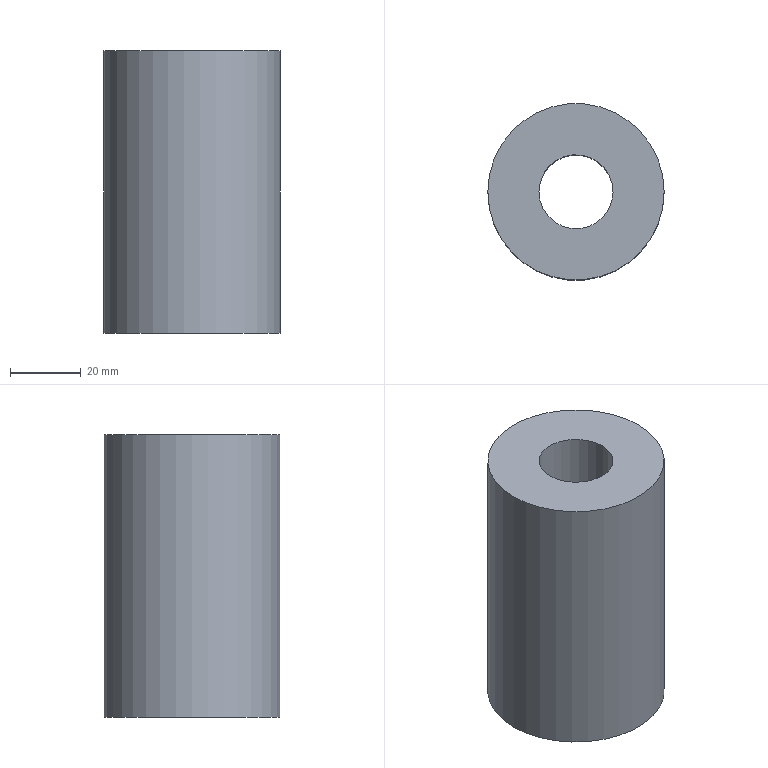Part | STEP file | SN10_014_002-02_TUBO | 1 solid | 4 faces | box 50 x 50 x 80 mm | volume 129371 mm3 | cylinder 2 | plane 2 | commonest cylinder face diameters 21 x1 50 x1
STEP:
#1=CARTESIAN_POINT('',(0.,0.,0.));
#2=DIRECTION('',(0.,0.,1.));
#3=DIRECTION('',(1.,0.,0.));
#4=AXIS2_PLACEMENT_3D('',#1,#2,#3);
#5=CARTESIAN_POINT('',(9.215,-5.034,92.5));
#6=VERTEX_POINT('',#5);
#7=CARTESIAN_POINT('',(0.,0.,92.5));
#8=DIRECTION('',(0.,0.,-1.));
#9=DIRECTION('',(1.,0.,0.));
#10=AXIS2_PLACEMENT_3D('',#7,#8,#9);
#11=CIRCLE('',#10,10.5);
#12=CARTESIAN_POINT('',(0.,0.,92.4));
#13=DIRECTION('',(0.,0.,-1.));
#14=DIRECTION('',(0.8776,-0.4794,0.));
#15=AXIS2_PLACEMENT_3D('',#12,#13,#14);
#16=CYLINDRICAL_SURFACE('',#15,10.5);
#17=CARTESIAN_POINT('',(-0.5,-0.1));
#18=DIRECTION('',(1.,0.));
#19=VECTOR('',#18,1.);
#20=LINE('',#17,#19);
#21=(GEOMETRIC_REPRESENTATION_CONTEXT(2)PARAMETRIC_REPRESENTATION_CONTEXT()REPRESENTATION_CONTEXT('',''));
#22=DEFINITIONAL_REPRESENTATION('',(#20),#21);
#23=PCURVE('',#16,#22);
#24=CARTESIAN_POINT('',(0.,0.,92.5));
#25=DIRECTION('',(0.,0.,-1.));
#26=DIRECTION('',(-1.,0.,0.));
#27=AXIS2_PLACEMENT_3D('',#24,#25,#26);
#28=PLANE('',#27);
#29=CARTESIAN_POINT('',(0.,0.));
#30=DIRECTION('',(-1.,0.));
#31=AXIS2_PLACEMENT_2D('',#29,#30);
#32=CIRCLE('',#31,10.5);
#33=(GEOMETRIC_REPRESENTATION_CONTEXT(2)PARAMETRIC_REPRESENTATION_CONTEXT()REPRESENTATION_CONTEXT('',''));
#34=DEFINITIONAL_REPRESENTATION('',(#32),#33);
#35=PCURVE('',#28,#34);
#36=SURFACE_CURVE('',#11,(#23,#35),.PCURVE_S1.);
#37=EDGE_CURVE('',#6,#6,#36,.T.);
#38=ORIENTED_EDGE('',*,*,#37,.T.);
#39=CARTESIAN_POINT('',(9.215,-5.034,12.5));
#40=VERTEX_POINT('',#39);
#41=CARTESIAN_POINT('',(9.215,-5.034,92.5));
#42=CARTESIAN_POINT('',(9.215,-5.034,12.5));
#43=B_SPLINE_CURVE_WITH_KNOTS('',1,(#41,#42),.UNSPECIFIED.,.F.,.F.,(2,2),(-0.1,79.9),.PIECEWISE_BEZIER_KNOTS.);
#44=CARTESIAN_POINT('',(6.283,0.));
#45=DIRECTION('',(0.,1.));
#46=VECTOR('',#45,1.);
#47=LINE('',#44,#46);
#48=(GEOMETRIC_REPRESENTATION_CONTEXT(2)PARAMETRIC_REPRESENTATION_CONTEXT()REPRESENTATION_CONTEXT('',''));
#49=DEFINITIONAL_REPRESENTATION('',(#47),#48);
#50=PCURVE('',#16,#49);
#51=CARTESIAN_POINT('',(0.,0.));
#52=DIRECTION('',(0.,1.));
#53=VECTOR('',#52,1.);
#54=LINE('',#51,#53);
#55=(GEOMETRIC_REPRESENTATION_CONTEXT(2)PARAMETRIC_REPRESENTATION_CONTEXT()REPRESENTATION_CONTEXT('',''));
#56=DEFINITIONAL_REPRESENTATION('',(#54),#55);
#57=PCURVE('',#16,#56);
#58=SEAM_CURVE('',#43,(#50,#57),.PCURVE_S1.);
#59=EDGE_CURVE('',#6,#40,#58,.T.);
#60=ORIENTED_EDGE('',*,*,#59,.T.);
#61=CARTESIAN_POINT('',(0.,0.,12.5));
#62=DIRECTION('',(0.,0.,-1.));
#63=DIRECTION('',(1.,0.,0.));
#64=AXIS2_PLACEMENT_3D('',#61,#62,#63);
#65=CIRCLE('',#64,10.5);
#66=CARTESIAN_POINT('',(-0.5,79.9));
#67=DIRECTION('',(1.,0.));
#68=VECTOR('',#67,1.);
#69=LINE('',#66,#68);
#70=(GEOMETRIC_REPRESENTATION_CONTEXT(2)PARAMETRIC_REPRESENTATION_CONTEXT()REPRESENTATION_CONTEXT('',''));
#71=DEFINITIONAL_REPRESENTATION('',(#69),#70);
#72=PCURVE('',#16,#71);
#73=CARTESIAN_POINT('',(0.,0.,12.5));
#74=DIRECTION('',(0.,0.,-1.));
#75=DIRECTION('',(-1.,0.,0.));
#76=AXIS2_PLACEMENT_3D('',#73,#74,#75);
#77=PLANE('',#76);
#78=CARTESIAN_POINT('',(0.,0.));
#79=DIRECTION('',(-1.,0.));
#80=AXIS2_PLACEMENT_2D('',#78,#79);
#81=CIRCLE('',#80,10.5);
#82=(GEOMETRIC_REPRESENTATION_CONTEXT(2)PARAMETRIC_REPRESENTATION_CONTEXT()REPRESENTATION_CONTEXT('',''));
#83=DEFINITIONAL_REPRESENTATION('',(#81),#82);
#84=PCURVE('',#77,#83);
#85=SURFACE_CURVE('',#65,(#72,#84),.PCURVE_S1.);
#86=EDGE_CURVE('',#40,#40,#85,.T.);
#87=ORIENTED_EDGE('',*,*,#86,.F.);
#88=ORIENTED_EDGE('',*,*,#59,.F.);
#89=EDGE_LOOP('',(#38,#60,#87,#88));
#90=FACE_BOUND('',#89,.F.);
#91=ADVANCED_FACE('',(#90),#16,.F.);
#92=CARTESIAN_POINT('',(25.,0.,12.5));
#93=VERTEX_POINT('',#92);
#94=CARTESIAN_POINT('',(0.,0.,12.5));
#95=DIRECTION('',(0.,0.,-1.));
#96=DIRECTION('',(1.,0.,0.));
#97=AXIS2_PLACEMENT_3D('',#94,#95,#96);
#98=CIRCLE('',#97,25.);
#99=CARTESIAN_POINT('',(0.,0.));
#100=DIRECTION('',(-1.,0.));
#101=AXIS2_PLACEMENT_2D('',#99,#100);
#102=CIRCLE('',#101,25.);
#103=(GEOMETRIC_REPRESENTATION_CONTEXT(2)PARAMETRIC_REPRESENTATION_CONTEXT()REPRESENTATION_CONTEXT('',''));
#104=DEFINITIONAL_REPRESENTATION('',(#102),#103);
#105=PCURVE('',#77,#104);
#106=CARTESIAN_POINT('',(0.,0.,52.5));
#107=DIRECTION('',(0.,0.,-1.));
#108=DIRECTION('',(1.,0.,0.));
#109=AXIS2_PLACEMENT_3D('',#106,#107,#108);
#110=CYLINDRICAL_SURFACE('',#109,25.);
#111=CARTESIAN_POINT('',(0.,40.));
#112=DIRECTION('',(1.,0.));
#113=VECTOR('',#112,1.);
#114=LINE('',#111,#113);
#115=(GEOMETRIC_REPRESENTATION_CONTEXT(2)PARAMETRIC_REPRESENTATION_CONTEXT()REPRESENTATION_CONTEXT('',''));
#116=DEFINITIONAL_REPRESENTATION('',(#114),#115);
#117=PCURVE('',#110,#116);
#118=SURFACE_CURVE('',#98,(#105,#117),.PCURVE_S1.);
#119=EDGE_CURVE('',#93,#93,#118,.T.);
#120=ORIENTED_EDGE('',*,*,#119,.T.);
#121=EDGE_LOOP('',(#120));
#122=FACE_BOUND('',#121,.T.);
#123=ORIENTED_EDGE('',*,*,#86,.F.);
#124=EDGE_LOOP('',(#123));
#125=FACE_BOUND('',#124,.T.);
#126=ADVANCED_FACE('',(#122,#125),#77,.T.);
#127=CARTESIAN_POINT('',(25.,0.,92.5));
#128=VERTEX_POINT('',#127);
#129=CARTESIAN_POINT('',(0.,0.,92.5));
#130=DIRECTION('',(0.,0.,-1.));
#131=DIRECTION('',(1.,0.,0.));
#132=AXIS2_PLACEMENT_3D('',#129,#130,#131);
#133=CIRCLE('',#132,25.);
#134=CARTESIAN_POINT('',(0.,-40.));
#135=DIRECTION('',(1.,0.));
#136=VECTOR('',#135,1.);
#137=LINE('',#134,#136);
#138=(GEOMETRIC_REPRESENTATION_CONTEXT(2)PARAMETRIC_REPRESENTATION_CONTEXT()REPRESENTATION_CONTEXT('',''));
#139=DEFINITIONAL_REPRESENTATION('',(#137),#138);
#140=PCURVE('',#110,#139);
#141=CARTESIAN_POINT('',(0.,0.));
#142=DIRECTION('',(-1.,0.));
#143=AXIS2_PLACEMENT_2D('',#141,#142);
#144=CIRCLE('',#143,25.);
#145=(GEOMETRIC_REPRESENTATION_CONTEXT(2)PARAMETRIC_REPRESENTATION_CONTEXT()REPRESENTATION_CONTEXT('',''));
#146=DEFINITIONAL_REPRESENTATION('',(#144),#145);
#147=PCURVE('',#28,#146);
#148=SURFACE_CURVE('',#133,(#140,#147),.PCURVE_S1.);
#149=EDGE_CURVE('',#128,#128,#148,.T.);
#150=ORIENTED_EDGE('',*,*,#149,.T.);
#151=CARTESIAN_POINT('',(25.,0.,92.5));
#152=CARTESIAN_POINT('',(25.,0.,12.5));
#153=B_SPLINE_CURVE_WITH_KNOTS('',1,(#151,#152),.UNSPECIFIED.,.F.,.F.,(2,2),(-40.,40.),.PIECEWISE_BEZIER_KNOTS.);
#154=CARTESIAN_POINT('',(6.283,0.));
#155=DIRECTION('',(0.,1.));
#156=VECTOR('',#155,1.);
#157=LINE('',#154,#156);
#158=(GEOMETRIC_REPRESENTATION_CONTEXT(2)PARAMETRIC_REPRESENTATION_CONTEXT()REPRESENTATION_CONTEXT('',''));
#159=DEFINITIONAL_REPRESENTATION('',(#157),#158);
#160=PCURVE('',#110,#159);
#161=CARTESIAN_POINT('',(0.,0.));
#162=DIRECTION('',(0.,1.));
#163=VECTOR('',#162,1.);
#164=LINE('',#161,#163);
#165=(GEOMETRIC_REPRESENTATION_CONTEXT(2)PARAMETRIC_REPRESENTATION_CONTEXT()REPRESENTATION_CONTEXT('',''));
#166=DEFINITIONAL_REPRESENTATION('',(#164),#165);
#167=PCURVE('',#110,#166);
#168=SEAM_CURVE('',#153,(#160,#167),.PCURVE_S1.);
#169=EDGE_CURVE('',#128,#93,#168,.T.);
#170=ORIENTED_EDGE('',*,*,#169,.T.);
#171=ORIENTED_EDGE('',*,*,#119,.F.);
#172=ORIENTED_EDGE('',*,*,#169,.F.);
#173=EDGE_LOOP('',(#150,#170,#171,#172));
#174=FACE_BOUND('',#173,.T.);
#175=ADVANCED_FACE('',(#174),#110,.T.);
#176=ORIENTED_EDGE('',*,*,#149,.F.);
#177=EDGE_LOOP('',(#176));
#178=FACE_BOUND('',#177,.T.);
#179=ORIENTED_EDGE('',*,*,#37,.T.);
#180=EDGE_LOOP('',(#179));
#181=FACE_BOUND('',#180,.T.);
#182=ADVANCED_FACE('',(#178,#181),#28,.F.);
#183=CLOSED_SHELL('',(#91,#126,#175,#182));
#184=MANIFOLD_SOLID_BREP('',#183);
#185=(LENGTH_UNIT()NAMED_UNIT(*)SI_UNIT(.MILLI.,.METRE.));
#186=UNCERTAINTY_MEASURE_WITH_UNIT(LENGTH_MEASURE(0.00001),#185,'','');
#187=(NAMED_UNIT(*)PLANE_ANGLE_UNIT()SI_UNIT($,.RADIAN.));
#188=(NAMED_UNIT(*)SI_UNIT($,.STERADIAN.)SOLID_ANGLE_UNIT());
#189=(GEOMETRIC_REPRESENTATION_CONTEXT(3)GLOBAL_UNCERTAINTY_ASSIGNED_CONTEXT((#186))GLOBAL_UNIT_ASSIGNED_CONTEXT((#185,#187,#188))REPRESENTATION_CONTEXT('',''));
#190=ADVANCED_BREP_SHAPE_REPRESENTATION('',(#4,#184),#189);